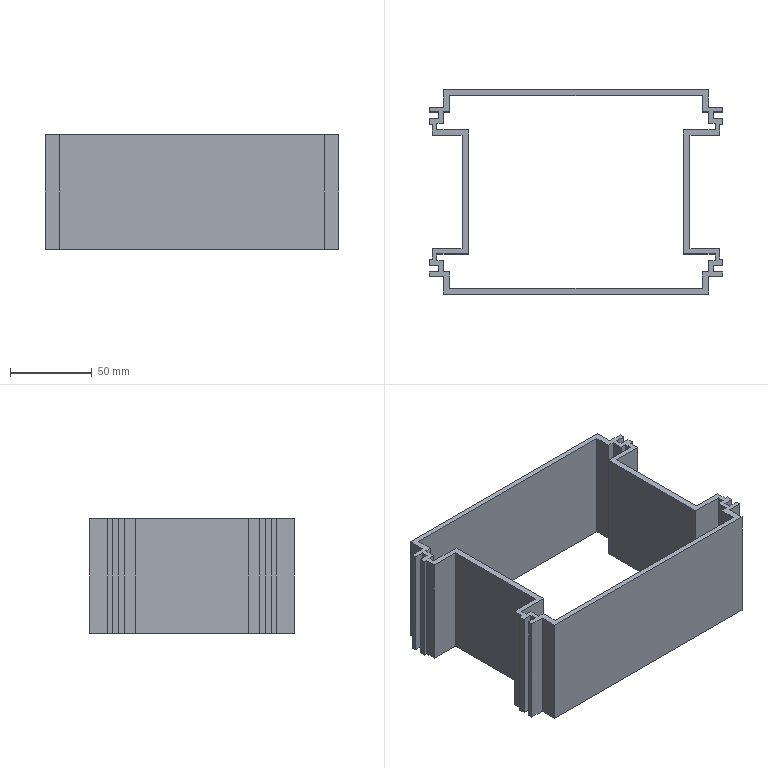Part | SolidWorks | features Extrusion 1 | 1 solid | 74 faces | box 180 x 125.252 x 70 mm | volume 170034 mm3 | plane 74